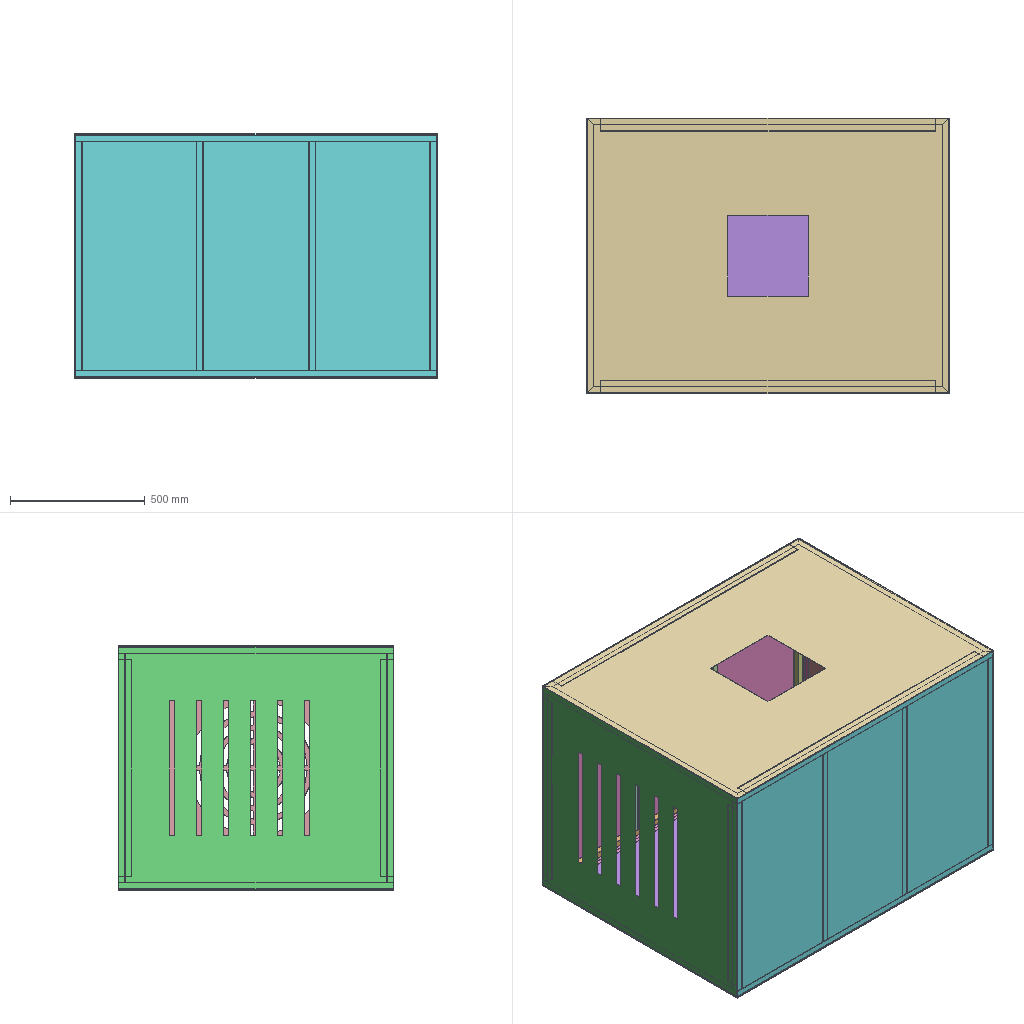Assembly | SolidWorks | 7 different items | 7 placed | box 1348 x 1022 x 907 mm
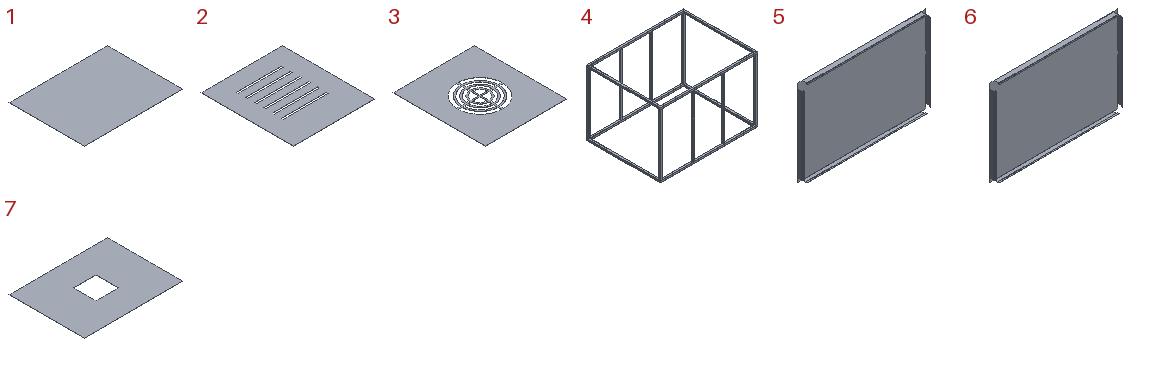Parts list (item | quantity | size | volume | features):
1 | x1 | 1345 x 1022 x 1.5 mm | 2062692 mm3 | features FlatPattern 1, SMBaseFlange 1, SheetMetal 1
2 | x1 | 904 x 1022 x 1.5 mm | 1296374 mm3 | features FlatPattern 1, SMBaseFlange 1, SheetMetal 1
3 | x1 | 904 x 1022 x 1.5 mm | 1198858 mm3 | features FlatPattern 1, MacroFeature 1, SMBaseFlange 1, SheetMetal 1
4 | x1 | 1341 x 1020 x 900 mm | 1809729 mm3 | features 3DProfileFeature 1, WeldMemberFeat 1, WeldmentFeature 1
5 | x1 | 1345 x 63.8 x 904 mm | 1806228 mm3 | features EdgeFlange 8, FlatPattern 1, SMBaseFlange 1, SheetMetal 1
6 | x1 | 1345 x 63.8 x 904 mm | 1806228 mm3 | features EdgeFlange 8, FlatPattern 1, SMBaseFlange 1, SheetMetal 1
7 | x1 | 1345 x 1022 x 1.5 mm | 1927692 mm3 | features FlatPattern 1, SMBaseFlange 1, SheetMetal 1
Mates (type | each side: item.copy, entity, surface, feature):
Coincident | 4.1 plane | 5.1 plane | 2 times
Coincident | 4.1 face plane Structural Member1 | 5.1 face plane Base-Flange1
Coincident | 5.1 plane | 6.1 plane | 2 times
Coincident | 4.1 face plane Structural Member1 | 6.1 face plane Base-Flange1
InPlace | 5.1 face plane Edge-Flange1 | 7.1 plane
InPlace | 5.1 face plane Edge-Flange1 | 1.1 plane
InPlace | 5.1 face plane Edge-Flange1 | 2.1 plane
InPlace | 5.1 face plane Edge-Flange1 | 3.1 plane